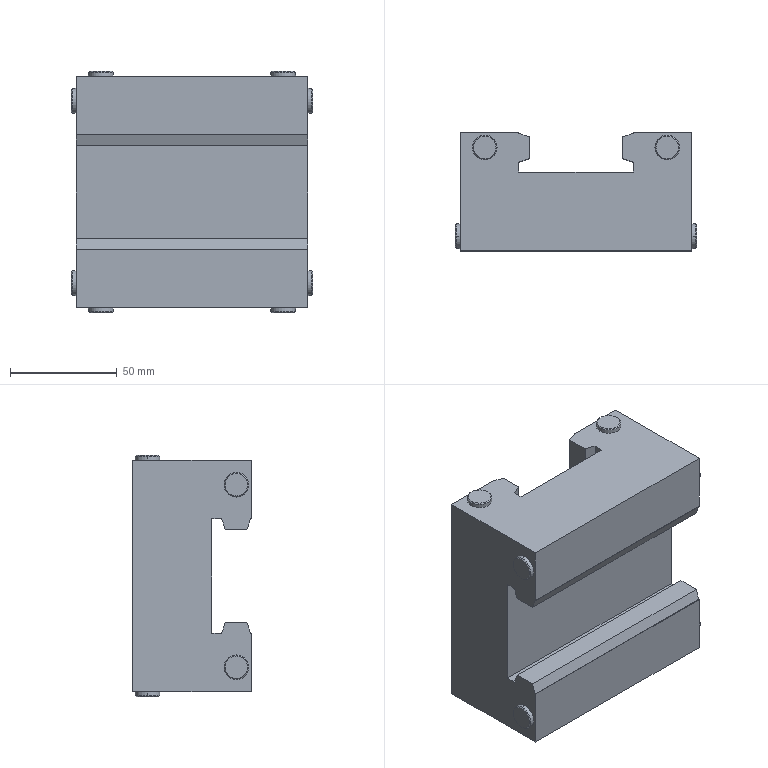Part | SolidWorks | features BaseBody 1 | 1 solid | 70 faces | box 113.077 x 55.385 x 113.077 mm | volume 463950 mm3 | plane 38 | cylinder 16 | cone 16 | commonest cylinder face diameters 11.538 x16